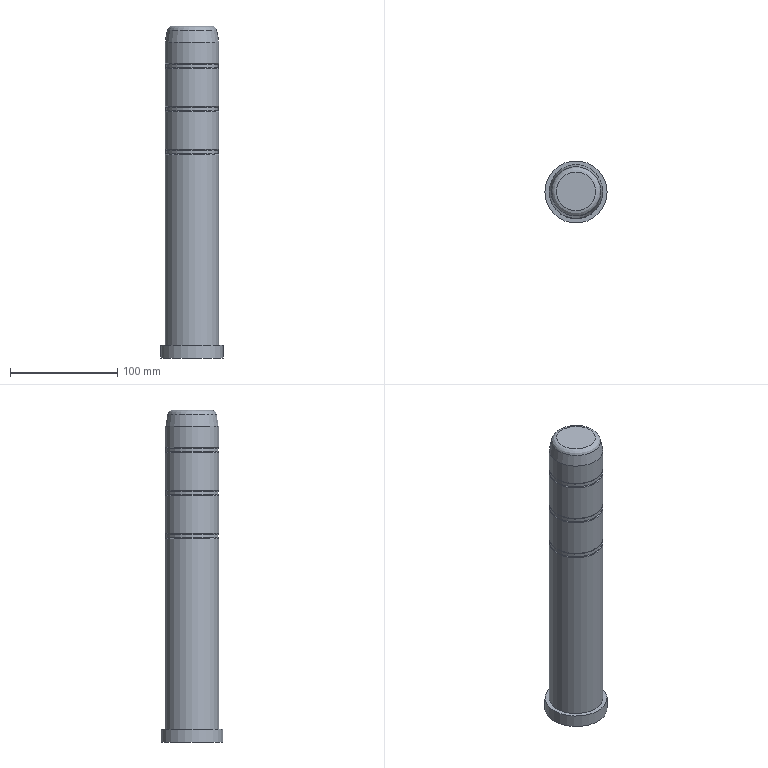Part | STEP file | GP50 | 1 solid | 19 faces | box 58 x 58 x 310 mm | volume 612293 mm3 | cylinder 8 | torus 7 | plane 3 | cone 1 | commonest cylinder face diameters 50 x4 49 x3 58 x1
STEP:
#1=CARTESIAN_POINT('',(0.,0.,0.));
#2=DIRECTION('',(0.,0.,1.));
#3=DIRECTION('',(1.,0.,0.));
#4=AXIS2_PLACEMENT_3D('',#1,#2,#3);
#5=CARTESIAN_POINT('',(247.,-268.,44.));
#6=VERTEX_POINT('',#5);
#7=CARTESIAN_POINT('',(222.,-268.,44.));
#8=DIRECTION('',(0.,0.,1.));
#9=DIRECTION('',(1.,0.,0.));
#10=AXIS2_PLACEMENT_3D('',#7,#8,#9);
#11=CIRCLE('',#10,25.);
#12=CARTESIAN_POINT('',(222.,-268.,534.));
#13=DIRECTION('',(0.,0.,-1.));
#14=DIRECTION('',(1.,0.,0.));
#15=AXIS2_PLACEMENT_3D('',#12,#13,#14);
#16=CYLINDRICAL_SURFACE('',#15,25.);
#17=CARTESIAN_POINT('',(6.283,490.));
#18=DIRECTION('',(-1.,0.));
#19=VECTOR('',#18,1.);
#20=LINE('',#17,#19);
#21=(GEOMETRIC_REPRESENTATION_CONTEXT(2)PARAMETRIC_REPRESENTATION_CONTEXT()REPRESENTATION_CONTEXT('',''));
#22=DEFINITIONAL_REPRESENTATION('',(#20),#21);
#23=PCURVE('',#16,#22);
#24=CARTESIAN_POINT('',(222.,-268.,43.134));
#25=DIRECTION('',(0.,0.,1.));
#26=DIRECTION('',(1.,0.,0.));
#27=AXIS2_PLACEMENT_3D('',#24,#25,#26);
#28=TOROIDAL_SURFACE('',#27,25.5,1.);
#29=CARTESIAN_POINT('',(0.,8.378));
#30=DIRECTION('',(1.,0.));
#31=VECTOR('',#30,1.);
#32=LINE('',#29,#31);
#33=(GEOMETRIC_REPRESENTATION_CONTEXT(2)PARAMETRIC_REPRESENTATION_CONTEXT()REPRESENTATION_CONTEXT('',''));
#34=DEFINITIONAL_REPRESENTATION('',(#32),#33);
#35=PCURVE('',#28,#34);
#36=SURFACE_CURVE('',#11,(#23,#35),.PCURVE_S1.);
#37=EDGE_CURVE('',#6,#6,#36,.T.);
#38=ORIENTED_EDGE('',*,*,#37,.T.);
#39=CARTESIAN_POINT('',(247.,-268.,79.));
#40=VERTEX_POINT('',#39);
#41=CARTESIAN_POINT('',(247.,-268.,79.));
#42=CARTESIAN_POINT('',(247.,-268.,44.));
#43=B_SPLINE_CURVE_WITH_KNOTS('',1,(#41,#42),.UNSPECIFIED.,.F.,.F.,(2,2),(455.,490.),.PIECEWISE_BEZIER_KNOTS.);
#44=CARTESIAN_POINT('',(0.,0.));
#45=DIRECTION('',(0.,1.));
#46=VECTOR('',#45,1.);
#47=LINE('',#44,#46);
#48=(GEOMETRIC_REPRESENTATION_CONTEXT(2)PARAMETRIC_REPRESENTATION_CONTEXT()REPRESENTATION_CONTEXT('',''));
#49=DEFINITIONAL_REPRESENTATION('',(#47),#48);
#50=PCURVE('',#16,#49);
#51=CARTESIAN_POINT('',(6.283,0.));
#52=DIRECTION('',(0.,1.));
#53=VECTOR('',#52,1.);
#54=LINE('',#51,#53);
#55=(GEOMETRIC_REPRESENTATION_CONTEXT(2)PARAMETRIC_REPRESENTATION_CONTEXT()REPRESENTATION_CONTEXT('',''));
#56=DEFINITIONAL_REPRESENTATION('',(#54),#55);
#57=PCURVE('',#16,#56);
#58=SEAM_CURVE('',#43,(#50,#57),.PCURVE_S1.);
#59=EDGE_CURVE('',#40,#6,#58,.T.);
#60=ORIENTED_EDGE('',*,*,#59,.F.);
#61=CARTESIAN_POINT('',(222.,-268.,79.));
#62=DIRECTION('',(0.,0.,1.));
#63=DIRECTION('',(1.,0.,0.));
#64=AXIS2_PLACEMENT_3D('',#61,#62,#63);
#65=CIRCLE('',#64,25.);
#66=CARTESIAN_POINT('',(6.283,455.));
#67=DIRECTION('',(-1.,0.));
#68=VECTOR('',#67,1.);
#69=LINE('',#66,#68);
#70=(GEOMETRIC_REPRESENTATION_CONTEXT(2)PARAMETRIC_REPRESENTATION_CONTEXT()REPRESENTATION_CONTEXT('',''));
#71=DEFINITIONAL_REPRESENTATION('',(#69),#70);
#72=PCURVE('',#16,#71);
#73=CARTESIAN_POINT('',(222.,-268.,79.866));
#74=DIRECTION('',(0.,0.,-1.));
#75=DIRECTION('',(-1.,0.,0.));
#76=AXIS2_PLACEMENT_3D('',#73,#74,#75);
#77=TOROIDAL_SURFACE('',#76,25.5,1.);
#78=CARTESIAN_POINT('',(9.425,8.378));
#79=DIRECTION('',(-1.,0.));
#80=VECTOR('',#79,1.);
#81=LINE('',#78,#80);
#82=(GEOMETRIC_REPRESENTATION_CONTEXT(2)PARAMETRIC_REPRESENTATION_CONTEXT()REPRESENTATION_CONTEXT('',''));
#83=DEFINITIONAL_REPRESENTATION('',(#81),#82);
#84=PCURVE('',#77,#83);
#85=SURFACE_CURVE('',#65,(#72,#84),.PCURVE_S1.);
#86=EDGE_CURVE('',#40,#40,#85,.T.);
#87=ORIENTED_EDGE('',*,*,#86,.F.);
#88=ORIENTED_EDGE('',*,*,#59,.T.);
#89=EDGE_LOOP('',(#38,#60,#87,#88));
#90=FACE_BOUND('',#89,.T.);
#91=ADVANCED_FACE('',(#90),#16,.T.);
#92=CARTESIAN_POINT('',(246.5,-268.,83.134));
#93=VERTEX_POINT('',#92);
#94=CARTESIAN_POINT('',(222.,-268.,83.134));
#95=DIRECTION('',(0.,0.,-1.));
#96=DIRECTION('',(1.,0.,0.));
#97=AXIS2_PLACEMENT_3D('',#94,#95,#96);
#98=CIRCLE('',#97,24.5);
#99=CARTESIAN_POINT('',(222.,-268.,534.));
#100=DIRECTION('',(0.,0.,-1.));
#101=DIRECTION('',(1.,0.,0.));
#102=AXIS2_PLACEMENT_3D('',#99,#100,#101);
#103=CYLINDRICAL_SURFACE('',#102,24.5);
#104=CARTESIAN_POINT('',(0.,450.866));
#105=DIRECTION('',(1.,0.));
#106=VECTOR('',#105,1.);
#107=LINE('',#104,#106);
#108=(GEOMETRIC_REPRESENTATION_CONTEXT(2)PARAMETRIC_REPRESENTATION_CONTEXT()REPRESENTATION_CONTEXT('',''));
#109=DEFINITIONAL_REPRESENTATION('',(#107),#108);
#110=PCURVE('',#103,#109);
#111=CARTESIAN_POINT('',(222.,-268.,83.134));
#112=DIRECTION('',(0.,0.,1.));
#113=DIRECTION('',(1.,0.,0.));
#114=AXIS2_PLACEMENT_3D('',#111,#112,#113);
#115=TOROIDAL_SURFACE('',#114,25.5,1.);
#116=CARTESIAN_POINT('',(6.283,9.425));
#117=DIRECTION('',(-1.,0.));
#118=VECTOR('',#117,1.);
#119=LINE('',#116,#118);
#120=(GEOMETRIC_REPRESENTATION_CONTEXT(2)PARAMETRIC_REPRESENTATION_CONTEXT()REPRESENTATION_CONTEXT('',''));
#121=DEFINITIONAL_REPRESENTATION('',(#119),#120);
#122=PCURVE('',#115,#121);
#123=SURFACE_CURVE('',#98,(#110,#122),.PCURVE_S1.);
#124=EDGE_CURVE('',#93,#93,#123,.T.);
#125=ORIENTED_EDGE('',*,*,#124,.T.);
#126=CARTESIAN_POINT('',(246.5,-268.,79.866));
#127=VERTEX_POINT('',#126);
#128=CARTESIAN_POINT('',(246.5,-268.,83.134));
#129=CARTESIAN_POINT('',(246.5,-268.,79.866));
#130=B_SPLINE_CURVE_WITH_KNOTS('',1,(#128,#129),.UNSPECIFIED.,.F.,.F.,(2,2),(450.866,454.134),.PIECEWISE_BEZIER_KNOTS.);
#131=CARTESIAN_POINT('',(6.283,0.));
#132=DIRECTION('',(0.,1.));
#133=VECTOR('',#132,1.);
#134=LINE('',#131,#133);
#135=(GEOMETRIC_REPRESENTATION_CONTEXT(2)PARAMETRIC_REPRESENTATION_CONTEXT()REPRESENTATION_CONTEXT('',''));
#136=DEFINITIONAL_REPRESENTATION('',(#134),#135);
#137=PCURVE('',#103,#136);
#138=CARTESIAN_POINT('',(0.,0.));
#139=DIRECTION('',(0.,1.));
#140=VECTOR('',#139,1.);
#141=LINE('',#138,#140);
#142=(GEOMETRIC_REPRESENTATION_CONTEXT(2)PARAMETRIC_REPRESENTATION_CONTEXT()REPRESENTATION_CONTEXT('',''));
#143=DEFINITIONAL_REPRESENTATION('',(#141),#142);
#144=PCURVE('',#103,#143);
#145=SEAM_CURVE('',#130,(#137,#144),.PCURVE_S1.);
#146=EDGE_CURVE('',#93,#127,#145,.T.);
#147=ORIENTED_EDGE('',*,*,#146,.T.);
#148=CARTESIAN_POINT('',(197.5,-268.,79.866));
#149=VERTEX_POINT('',#148);
#150=CARTESIAN_POINT('',(222.,-268.,79.866));
#151=DIRECTION('',(0.,0.,1.));
#152=DIRECTION('',(-1.,0.,0.));
#153=AXIS2_PLACEMENT_3D('',#150,#151,#152);
#154=CIRCLE('',#153,24.5);
#155=CARTESIAN_POINT('',(9.425,454.134));
#156=DIRECTION('',(-1.,0.));
#157=VECTOR('',#156,1.);
#158=LINE('',#155,#157);
#159=(GEOMETRIC_REPRESENTATION_CONTEXT(2)PARAMETRIC_REPRESENTATION_CONTEXT()REPRESENTATION_CONTEXT('',''));
#160=DEFINITIONAL_REPRESENTATION('',(#158),#159);
#161=PCURVE('',#103,#160);
#162=CARTESIAN_POINT('',(12.566,9.425));
#163=DIRECTION('',(-1.,0.));
#164=VECTOR('',#163,1.);
#165=LINE('',#162,#164);
#166=(GEOMETRIC_REPRESENTATION_CONTEXT(2)PARAMETRIC_REPRESENTATION_CONTEXT()REPRESENTATION_CONTEXT('',''));
#167=DEFINITIONAL_REPRESENTATION('',(#165),#166);
#168=PCURVE('',#77,#167);
#169=SURFACE_CURVE('',#154,(#161,#168),.PCURVE_S1.);
#170=EDGE_CURVE('',#127,#149,#169,.T.);
#171=ORIENTED_EDGE('',*,*,#170,.T.);
#172=CARTESIAN_POINT('',(222.,-268.,79.866));
#173=DIRECTION('',(0.,0.,1.));
#174=DIRECTION('',(-1.,0.,0.));
#175=AXIS2_PLACEMENT_3D('',#172,#173,#174);
#176=CIRCLE('',#175,24.5);
#177=CARTESIAN_POINT('',(3.142,454.134));
#178=DIRECTION('',(-1.,0.));
#179=VECTOR('',#178,1.);
#180=LINE('',#177,#179);
#181=(GEOMETRIC_REPRESENTATION_CONTEXT(2)PARAMETRIC_REPRESENTATION_CONTEXT()REPRESENTATION_CONTEXT('',''));
#182=DEFINITIONAL_REPRESENTATION('',(#180),#181);
#183=PCURVE('',#103,#182);
#184=CARTESIAN_POINT('',(6.283,9.425));
#185=DIRECTION('',(-1.,0.));
#186=VECTOR('',#185,1.);
#187=LINE('',#184,#186);
#188=(GEOMETRIC_REPRESENTATION_CONTEXT(2)PARAMETRIC_REPRESENTATION_CONTEXT()REPRESENTATION_CONTEXT('',''));
#189=DEFINITIONAL_REPRESENTATION('',(#187),#188);
#190=PCURVE('',#77,#189);
#191=SURFACE_CURVE('',#176,(#183,#190),.PCURVE_S1.);
#192=EDGE_CURVE('',#149,#127,#191,.T.);
#193=ORIENTED_EDGE('',*,*,#192,.T.);
#194=ORIENTED_EDGE('',*,*,#146,.F.);
#195=EDGE_LOOP('',(#125,#147,#171,#193,#194));
#196=FACE_BOUND('',#195,.T.);
#197=ADVANCED_FACE('',(#196),#103,.T.);
#198=CARTESIAN_POINT('',(246.5,-268.,123.134));
#199=VERTEX_POINT('',#198);
#200=CARTESIAN_POINT('',(222.,-268.,123.134));
#201=DIRECTION('',(0.,0.,-1.));
#202=DIRECTION('',(1.,0.,0.));
#203=AXIS2_PLACEMENT_3D('',#200,#201,#202);
#204=CIRCLE('',#203,24.5);
#205=CARTESIAN_POINT('',(222.,-268.,534.));
#206=DIRECTION('',(0.,0.,-1.));
#207=DIRECTION('',(1.,0.,0.));
#208=AXIS2_PLACEMENT_3D('',#205,#206,#207);
#209=CYLINDRICAL_SURFACE('',#208,24.5);
#210=CARTESIAN_POINT('',(0.,410.866));
#211=DIRECTION('',(1.,0.));
#212=VECTOR('',#211,1.);
#213=LINE('',#210,#212);
#214=(GEOMETRIC_REPRESENTATION_CONTEXT(2)PARAMETRIC_REPRESENTATION_CONTEXT()REPRESENTATION_CONTEXT('',''));
#215=DEFINITIONAL_REPRESENTATION('',(#213),#214);
#216=PCURVE('',#209,#215);
#217=CARTESIAN_POINT('',(222.,-268.,123.134));
#218=DIRECTION('',(0.,0.,1.));
#219=DIRECTION('',(1.,0.,0.));
#220=AXIS2_PLACEMENT_3D('',#217,#218,#219);
#221=TOROIDAL_SURFACE('',#220,25.5,1.);
#222=CARTESIAN_POINT('',(6.283,9.425));
#223=DIRECTION('',(-1.,0.));
#224=VECTOR('',#223,1.);
#225=LINE('',#222,#224);
#226=(GEOMETRIC_REPRESENTATION_CONTEXT(2)PARAMETRIC_REPRESENTATION_CONTEXT()REPRESENTATION_CONTEXT('',''));
#227=DEFINITIONAL_REPRESENTATION('',(#225),#226);
#228=PCURVE('',#221,#227);
#229=SURFACE_CURVE('',#204,(#216,#228),.PCURVE_S1.);
#230=EDGE_CURVE('',#199,#199,#229,.T.);
#231=ORIENTED_EDGE('',*,*,#230,.T.);
#232=CARTESIAN_POINT('',(246.5,-268.,119.866));
#233=VERTEX_POINT('',#232);
#234=CARTESIAN_POINT('',(246.5,-268.,123.134));
#235=CARTESIAN_POINT('',(246.5,-268.,119.866));
#236=B_SPLINE_CURVE_WITH_KNOTS('',1,(#234,#235),.UNSPECIFIED.,.F.,.F.,(2,2),(410.866,414.134),.PIECEWISE_BEZIER_KNOTS.);
#237=CARTESIAN_POINT('',(6.283,0.));
#238=DIRECTION('',(0.,1.));
#239=VECTOR('',#238,1.);
#240=LINE('',#237,#239);
#241=(GEOMETRIC_REPRESENTATION_CONTEXT(2)PARAMETRIC_REPRESENTATION_CONTEXT()REPRESENTATION_CONTEXT('',''));
#242=DEFINITIONAL_REPRESENTATION('',(#240),#241);
#243=PCURVE('',#209,#242);
#244=CARTESIAN_POINT('',(0.,0.));
#245=DIRECTION('',(0.,1.));
#246=VECTOR('',#245,1.);
#247=LINE('',#244,#246);
#248=(GEOMETRIC_REPRESENTATION_CONTEXT(2)PARAMETRIC_REPRESENTATION_CONTEXT()REPRESENTATION_CONTEXT('',''));
#249=DEFINITIONAL_REPRESENTATION('',(#247),#248);
#250=PCURVE('',#209,#249);
#251=SEAM_CURVE('',#236,(#243,#250),.PCURVE_S1.);
#252=EDGE_CURVE('',#199,#233,#251,.T.);
#253=ORIENTED_EDGE('',*,*,#252,.T.);
#254=CARTESIAN_POINT('',(197.5,-268.,119.866));
#255=VERTEX_POINT('',#254);
#256=CARTESIAN_POINT('',(222.,-268.,119.866));
#257=DIRECTION('',(0.,0.,1.));
#258=DIRECTION('',(-1.,0.,0.));
#259=AXIS2_PLACEMENT_3D('',#256,#257,#258);
#260=CIRCLE('',#259,24.5);
#261=CARTESIAN_POINT('',(9.425,414.134));
#262=DIRECTION('',(-1.,0.));
#263=VECTOR('',#262,1.);
#264=LINE('',#261,#263);
#265=(GEOMETRIC_REPRESENTATION_CONTEXT(2)PARAMETRIC_REPRESENTATION_CONTEXT()REPRESENTATION_CONTEXT('',''));
#266=DEFINITIONAL_REPRESENTATION('',(#264),#265);
#267=PCURVE('',#209,#266);
#268=CARTESIAN_POINT('',(222.,-268.,119.866));
#269=DIRECTION('',(0.,0.,-1.));
#270=DIRECTION('',(-1.,0.,0.));
#271=AXIS2_PLACEMENT_3D('',#268,#269,#270);
#272=TOROIDAL_SURFACE('',#271,25.5,1.);
#273=CARTESIAN_POINT('',(12.566,9.425));
#274=DIRECTION('',(-1.,0.));
#275=VECTOR('',#274,1.);
#276=LINE('',#273,#275);
#277=(GEOMETRIC_REPRESENTATION_CONTEXT(2)PARAMETRIC_REPRESENTATION_CONTEXT()REPRESENTATION_CONTEXT('',''));
#278=DEFINITIONAL_REPRESENTATION('',(#276),#277);
#279=PCURVE('',#272,#278);
#280=SURFACE_CURVE('',#260,(#267,#279),.PCURVE_S1.);
#281=EDGE_CURVE('',#233,#255,#280,.T.);
#282=ORIENTED_EDGE('',*,*,#281,.T.);
#283=CARTESIAN_POINT('',(222.,-268.,119.866));
#284=DIRECTION('',(0.,0.,1.));
#285=DIRECTION('',(-1.,0.,0.));
#286=AXIS2_PLACEMENT_3D('',#283,#284,#285);
#287=CIRCLE('',#286,24.5);
#288=CARTESIAN_POINT('',(3.142,414.134));
#289=DIRECTION('',(-1.,0.));
#290=VECTOR('',#289,1.);
#291=LINE('',#288,#290);
#292=(GEOMETRIC_REPRESENTATION_CONTEXT(2)PARAMETRIC_REPRESENTATION_CONTEXT()REPRESENTATION_CONTEXT('',''));
#293=DEFINITIONAL_REPRESENTATION('',(#291),#292);
#294=PCURVE('',#209,#293);
#295=CARTESIAN_POINT('',(6.283,9.425));
#296=DIRECTION('',(-1.,0.));
#297=VECTOR('',#296,1.);
#298=LINE('',#295,#297);
#299=(GEOMETRIC_REPRESENTATION_CONTEXT(2)PARAMETRIC_REPRESENTATION_CONTEXT()REPRESENTATION_CONTEXT('',''));
#300=DEFINITIONAL_REPRESENTATION('',(#298),#299);
#301=PCURVE('',#272,#300);
#302=SURFACE_CURVE('',#287,(#294,#301),.PCURVE_S1.);
#303=EDGE_CURVE('',#255,#233,#302,.T.);
#304=ORIENTED_EDGE('',*,*,#303,.T.);
#305=ORIENTED_EDGE('',*,*,#252,.F.);
#306=EDGE_LOOP('',(#231,#253,#282,#304,#305));
#307=FACE_BOUND('',#306,.T.);
#308=ADVANCED_FACE('',(#307),#209,.T.);
#309=CARTESIAN_POINT('',(203.84,-268.,159.));
#310=VERTEX_POINT('',#309);
#311=CARTESIAN_POINT('',(222.,-268.,159.));
#312=DIRECTION('',(0.,0.,1.));
#313=DIRECTION('',(-1.,0.,0.));
#314=AXIS2_PLACEMENT_3D('',#311,#312,#313);
#315=CIRCLE('',#314,18.16);
#316=CARTESIAN_POINT('',(-222.,272.,159.));
#317=DIRECTION('',(0.,0.,-1.));
#318=DIRECTION('',(1.,0.,0.));
#319=AXIS2_PLACEMENT_3D('',#316,#317,#318);
#320=PLANE('',#319);
#321=CARTESIAN_POINT('',(425.84,540.));
#322=CARTESIAN_POINT('',(425.84,571.453));
#323=CARTESIAN_POINT('',(453.08,555.727));
#324=CARTESIAN_POINT('',(480.319,540.));
#325=CARTESIAN_POINT('',(453.08,524.273));
#326=CARTESIAN_POINT('',(425.84,508.547));
#327=CARTESIAN_POINT('',(425.84,540.));
#328=(BOUNDED_CURVE()B_SPLINE_CURVE(2,(#321,#322,#323,#324,#325,#326,#327),.UNSPECIFIED.,.T.,.F.)B_SPLINE_CURVE_WITH_KNOTS((1,2,2,2,2,1),(-2.094,0.,2.094,4.189,6.283,8.378),.UNSPECIFIED.)CURVE()GEOMETRIC_REPRESENTATION_ITEM()RATIONAL_B_SPLINE_CURVE((1.,0.5,1.,0.5,1.,0.5,1.))REPRESENTATION_ITEM(''));
#329=(GEOMETRIC_REPRESENTATION_CONTEXT(2)PARAMETRIC_REPRESENTATION_CONTEXT()REPRESENTATION_CONTEXT('',''));
#330=DEFINITIONAL_REPRESENTATION('',(#328),#329);
#331=PCURVE('',#320,#330);
#332=CARTESIAN_POINT('',(222.,-268.,154.));
#333=DIRECTION('',(0.,0.,-1.));
#334=DIRECTION('',(-1.,0.,0.));
#335=AXIS2_PLACEMENT_3D('',#332,#333,#334);
#336=TOROIDAL_SURFACE('',#335,18.16,5.);
#337=CARTESIAN_POINT('',(6.283,4.712));
#338=DIRECTION('',(-1.,0.));
#339=VECTOR('',#338,1.);
#340=LINE('',#337,#339);
#341=(GEOMETRIC_REPRESENTATION_CONTEXT(2)PARAMETRIC_REPRESENTATION_CONTEXT()REPRESENTATION_CONTEXT('',''));
#342=DEFINITIONAL_REPRESENTATION('',(#340),#341);
#343=PCURVE('',#336,#342);
#344=SURFACE_CURVE('',#315,(#331,#343),.PCURVE_S1.);
#345=EDGE_CURVE('',#310,#310,#344,.T.);
#346=ORIENTED_EDGE('',*,*,#345,.T.);
#347=EDGE_LOOP('',(#346));
#348=FACE_BOUND('',#347,.T.);
#349=ADVANCED_FACE('',(#348),#320,.F.);
#350=CARTESIAN_POINT('',(198.916,-268.,154.868));
#351=VERTEX_POINT('',#350);
#352=CARTESIAN_POINT('',(222.,-268.,154.868));
#353=DIRECTION('',(0.,0.,-1.));
#354=DIRECTION('',(-1.,0.,0.));
#355=AXIS2_PLACEMENT_3D('',#352,#353,#354);
#356=CIRCLE('',#355,23.084);
#357=CARTESIAN_POINT('',(0.,6.109));
#358=DIRECTION('',(1.,0.));
#359=VECTOR('',#358,1.);
#360=LINE('',#357,#359);
#361=(GEOMETRIC_REPRESENTATION_CONTEXT(2)PARAMETRIC_REPRESENTATION_CONTEXT()REPRESENTATION_CONTEXT('',''));
#362=DEFINITIONAL_REPRESENTATION('',(#360),#361);
#363=PCURVE('',#336,#362);
#364=CARTESIAN_POINT('',(222.,-268.,159.));
#365=DIRECTION('',(0.,0.,-1.));
#366=DIRECTION('',(-1.,0.,0.));
#367=AXIS2_PLACEMENT_3D('',#364,#365,#366);
#368=CONICAL_SURFACE('',#367,22.355,0.1745);
#369=CARTESIAN_POINT('',(0.,4.132));
#370=DIRECTION('',(1.,0.));
#371=VECTOR('',#370,1.);
#372=LINE('',#369,#371);
#373=(GEOMETRIC_REPRESENTATION_CONTEXT(2)PARAMETRIC_REPRESENTATION_CONTEXT()REPRESENTATION_CONTEXT('',''));
#374=DEFINITIONAL_REPRESENTATION('',(#372),#373);
#375=PCURVE('',#368,#374);
#376=SURFACE_CURVE('',#356,(#363,#375),.PCURVE_S1.);
#377=EDGE_CURVE('',#351,#351,#376,.T.);
#378=ORIENTED_EDGE('',*,*,#377,.F.);
#379=CARTESIAN_POINT('',(203.84,-268.,159.));
#380=CARTESIAN_POINT('',(202.658,-268.,159.));
#381=CARTESIAN_POINT('',(201.499,-268.,158.667));
#382=CARTESIAN_POINT('',(200.466,-268.,158.021));
#383=CARTESIAN_POINT('',(199.651,-268.,157.116));
#384=CARTESIAN_POINT('',(199.122,-268.,156.033));
#385=CARTESIAN_POINT('',(198.916,-268.,154.868));
#386=(BOUNDED_CURVE()B_SPLINE_CURVE(6,(#379,#380,#381,#382,#383,#384,#385),.UNSPECIFIED.,.F.,.F.)B_SPLINE_CURVE_WITH_KNOTS((7,7),(4.712,6.109),.PIECEWISE_BEZIER_KNOTS.)CURVE()GEOMETRIC_REPRESENTATION_ITEM()RATIONAL_B_SPLINE_CURVE((1.025,1.008,0.9984,0.9952,0.9984,1.008,1.025))REPRESENTATION_ITEM(''));
#387=CARTESIAN_POINT('',(0.,0.));
#388=DIRECTION('',(0.,1.));
#389=VECTOR('',#388,1.);
#390=LINE('',#387,#389);
#391=(GEOMETRIC_REPRESENTATION_CONTEXT(2)PARAMETRIC_REPRESENTATION_CONTEXT()REPRESENTATION_CONTEXT('',''));
#392=DEFINITIONAL_REPRESENTATION('',(#390),#391);
#393=PCURVE('',#336,#392);
#394=CARTESIAN_POINT('',(6.283,0.));
#395=DIRECTION('',(0.,1.));
#396=VECTOR('',#395,1.);
#397=LINE('',#394,#396);
#398=(GEOMETRIC_REPRESENTATION_CONTEXT(2)PARAMETRIC_REPRESENTATION_CONTEXT()REPRESENTATION_CONTEXT('',''));
#399=DEFINITIONAL_REPRESENTATION('',(#397),#398);
#400=PCURVE('',#336,#399);
#401=SEAM_CURVE('',#386,(#393,#400),.PCURVE_S1.);
#402=EDGE_CURVE('',#310,#351,#401,.T.);
#403=ORIENTED_EDGE('',*,*,#402,.F.);
#404=ORIENTED_EDGE('',*,*,#345,.F.);
#405=ORIENTED_EDGE('',*,*,#402,.T.);
#406=EDGE_LOOP('',(#378,#403,#404,#405));
#407=FACE_BOUND('',#406,.T.);
#408=ADVANCED_FACE('',(#407),#336,.T.);
#409=ORIENTED_EDGE('',*,*,#377,.T.);
#410=CARTESIAN_POINT('',(197.,-268.,144.));
#411=VERTEX_POINT('',#410);
#412=CARTESIAN_POINT('',(198.916,-268.,154.868));
#413=CARTESIAN_POINT('',(197.,-268.,144.));
#414=B_SPLINE_CURVE_WITH_KNOTS('',1,(#412,#413),.UNSPECIFIED.,.F.,.F.,(2,2),(4.195,15.231),.PIECEWISE_BEZIER_KNOTS.);
#415=CARTESIAN_POINT('',(6.283,0.));
#416=DIRECTION('',(0.,1.));
#417=VECTOR('',#416,1.);
#418=LINE('',#415,#417);
#419=(GEOMETRIC_REPRESENTATION_CONTEXT(2)PARAMETRIC_REPRESENTATION_CONTEXT()REPRESENTATION_CONTEXT('',''));
#420=DEFINITIONAL_REPRESENTATION('',(#418),#419);
#421=PCURVE('',#368,#420);
#422=CARTESIAN_POINT('',(0.,0.));
#423=DIRECTION('',(0.,1.));
#424=VECTOR('',#423,1.);
#425=LINE('',#422,#424);
#426=(GEOMETRIC_REPRESENTATION_CONTEXT(2)PARAMETRIC_REPRESENTATION_CONTEXT()REPRESENTATION_CONTEXT('',''));
#427=DEFINITIONAL_REPRESENTATION('',(#425),#426);
#428=PCURVE('',#368,#427);
#429=SEAM_CURVE('',#414,(#421,#428),.PCURVE_S1.);
#430=EDGE_CURVE('',#351,#411,#429,.T.);
#431=ORIENTED_EDGE('',*,*,#430,.T.);
#432=CARTESIAN_POINT('',(247.,-268.,144.));
#433=VERTEX_POINT('',#432);
#434=CARTESIAN_POINT('',(222.,-268.,144.));
#435=DIRECTION('',(0.,0.,-1.));
#436=DIRECTION('',(-1.,0.,0.));
#437=AXIS2_PLACEMENT_3D('',#434,#435,#436);
#438=CIRCLE('',#437,25.);
#439=CARTESIAN_POINT('',(0.,15.));
#440=DIRECTION('',(1.,0.));
#441=VECTOR('',#440,1.);
#442=LINE('',#439,#441);
#443=(GEOMETRIC_REPRESENTATION_CONTEXT(2)PARAMETRIC_REPRESENTATION_CONTEXT()REPRESENTATION_CONTEXT('',''));
#444=DEFINITIONAL_REPRESENTATION('',(#442),#443);
#445=PCURVE('',#368,#444);
#446=CARTESIAN_POINT('',(222.,-268.,534.));
#447=DIRECTION('',(0.,0.,-1.));
#448=DIRECTION('',(1.,0.,0.));
#449=AXIS2_PLACEMENT_3D('',#446,#447,#448);
#450=CYLINDRICAL_SURFACE('',#449,25.);
#451=CARTESIAN_POINT('',(-3.142,390.));
#452=DIRECTION('',(1.,0.));
#453=VECTOR('',#452,1.);
#454=LINE('',#451,#453);
#455=(GEOMETRIC_REPRESENTATION_CONTEXT(2)PARAMETRIC_REPRESENTATION_CONTEXT()REPRESENTATION_CONTEXT('',''));
#456=DEFINITIONAL_REPRESENTATION('',(#454),#455);
#457=PCURVE('',#450,#456);
#458=SURFACE_CURVE('',#438,(#445,#457),.PCURVE_S1.);
#459=EDGE_CURVE('',#433,#411,#458,.T.);
#460=ORIENTED_EDGE('',*,*,#459,.F.);
#461=CARTESIAN_POINT('',(222.,-268.,144.));
#462=DIRECTION('',(0.,0.,-1.));
#463=DIRECTION('',(-1.,0.,0.));
#464=AXIS2_PLACEMENT_3D('',#461,#462,#463);
#465=CIRCLE('',#464,25.);
#466=CARTESIAN_POINT('',(0.,15.));
#467=DIRECTION('',(1.,0.));
#468=VECTOR('',#467,1.);
#469=LINE('',#466,#468);
#470=(GEOMETRIC_REPRESENTATION_CONTEXT(2)PARAMETRIC_REPRESENTATION_CONTEXT()REPRESENTATION_CONTEXT('',''));
#471=DEFINITIONAL_REPRESENTATION('',(#469),#470);
#472=PCURVE('',#368,#471);
#473=CARTESIAN_POINT('',(3.142,390.));
#474=DIRECTION('',(1.,0.));
#475=VECTOR('',#474,1.);
#476=LINE('',#473,#475);
#477=(GEOMETRIC_REPRESENTATION_CONTEXT(2)PARAMETRIC_REPRESENTATION_CONTEXT()REPRESENTATION_CONTEXT('',''));
#478=DEFINITIONAL_REPRESENTATION('',(#476),#477);
#479=PCURVE('',#450,#478);
#480=SURFACE_CURVE('',#465,(#472,#479),.PCURVE_S1.);
#481=EDGE_CURVE('',#411,#433,#480,.T.);
#482=ORIENTED_EDGE('',*,*,#481,.F.);
#483=ORIENTED_EDGE('',*,*,#430,.F.);
#484=EDGE_LOOP('',(#409,#431,#460,#482,#483));
#485=FACE_BOUND('',#484,.T.);
#486=ADVANCED_FACE('',(#485),#368,.T.);
#487=CARTESIAN_POINT('',(247.,-268.,124.));
#488=VERTEX_POINT('',#487);
#489=CARTESIAN_POINT('',(222.,-268.,124.));
#490=DIRECTION('',(0.,0.,1.));
#491=DIRECTION('',(1.,0.,0.));
#492=AXIS2_PLACEMENT_3D('',#489,#490,#491);
#493=CIRCLE('',#492,25.);
#494=CARTESIAN_POINT('',(6.283,410.));
#495=DIRECTION('',(-1.,0.));
#496=VECTOR('',#495,1.);
#497=LINE('',#494,#496);
#498=(GEOMETRIC_REPRESENTATION_CONTEXT(2)PARAMETRIC_REPRESENTATION_CONTEXT()REPRESENTATION_CONTEXT('',''));
#499=DEFINITIONAL_REPRESENTATION('',(#497),#498);
#500=PCURVE('',#450,#499);
#501=CARTESIAN_POINT('',(0.,8.378));
#502=DIRECTION('',(1.,0.));
#503=VECTOR('',#502,1.);
#504=LINE('',#501,#503);
#505=(GEOMETRIC_REPRESENTATION_CONTEXT(2)PARAMETRIC_REPRESENTATION_CONTEXT()REPRESENTATION_CONTEXT('',''));
#506=DEFINITIONAL_REPRESENTATION('',(#504),#505);
#507=PCURVE('',#221,#506);
#508=SURFACE_CURVE('',#493,(#500,#507),.PCURVE_S1.);
#509=EDGE_CURVE('',#488,#488,#508,.T.);
#510=ORIENTED_EDGE('',*,*,#509,.T.);
#511=CARTESIAN_POINT('',(247.,-268.,144.));
#512=CARTESIAN_POINT('',(247.,-268.,124.));
#513=B_SPLINE_CURVE_WITH_KNOTS('',1,(#511,#512),.UNSPECIFIED.,.F.,.F.,(2,2),(390.,410.),.PIECEWISE_BEZIER_KNOTS.);
#514=CARTESIAN_POINT('',(0.,0.));
#515=DIRECTION('',(0.,1.));
#516=VECTOR('',#515,1.);
#517=LINE('',#514,#516);
#518=(GEOMETRIC_REPRESENTATION_CONTEXT(2)PARAMETRIC_REPRESENTATION_CONTEXT()REPRESENTATION_CONTEXT('',''));
#519=DEFINITIONAL_REPRESENTATION('',(#517),#518);
#520=PCURVE('',#450,#519);
#521=CARTESIAN_POINT('',(6.283,0.));
#522=DIRECTION('',(0.,1.));
#523=VECTOR('',#522,1.);
#524=LINE('',#521,#523);
#525=(GEOMETRIC_REPRESENTATION_CONTEXT(2)PARAMETRIC_REPRESENTATION_CONTEXT()REPRESENTATION_CONTEXT('',''));
#526=DEFINITIONAL_REPRESENTATION('',(#524),#525);
#527=PCURVE('',#450,#526);
#528=SEAM_CURVE('',#513,(#520,#527),.PCURVE_S1.);
#529=EDGE_CURVE('',#433,#488,#528,.T.);
#530=ORIENTED_EDGE('',*,*,#529,.F.);
#531=ORIENTED_EDGE('',*,*,#459,.T.);
#532=ORIENTED_EDGE('',*,*,#481,.T.);
#533=ORIENTED_EDGE('',*,*,#529,.T.);
#534=EDGE_LOOP('',(#510,#530,#531,#532,#533));
#535=FACE_BOUND('',#534,.T.);
#536=ADVANCED_FACE('',(#535),#450,.T.);
#537=CARTESIAN_POINT('',(247.,-268.,84.));
#538=VERTEX_POINT('',#537);
#539=CARTESIAN_POINT('',(222.,-268.,84.));
#540=DIRECTION('',(0.,0.,1.));
#541=DIRECTION('',(1.,0.,0.));
#542=AXIS2_PLACEMENT_3D('',#539,#540,#541);
#543=CIRCLE('',#542,25.);
#544=CARTESIAN_POINT('',(222.,-268.,534.));
#545=DIRECTION('',(0.,0.,-1.));
#546=DIRECTION('',(1.,0.,0.));
#547=AXIS2_PLACEMENT_3D('',#544,#545,#546);
#548=CYLINDRICAL_SURFACE('',#547,25.);
#549=CARTESIAN_POINT('',(6.283,450.));
#550=DIRECTION('',(-1.,0.));
#551=VECTOR('',#550,1.);
#552=LINE('',#549,#551);
#553=(GEOMETRIC_REPRESENTATION_CONTEXT(2)PARAMETRIC_REPRESENTATION_CONTEXT()REPRESENTATION_CONTEXT('',''));
#554=DEFINITIONAL_REPRESENTATION('',(#552),#553);
#555=PCURVE('',#548,#554);
#556=CARTESIAN_POINT('',(0.,8.378));
#557=DIRECTION('',(1.,0.));
#558=VECTOR('',#557,1.);
#559=LINE('',#556,#558);
#560=(GEOMETRIC_REPRESENTATION_CONTEXT(2)PARAMETRIC_REPRESENTATION_CONTEXT()REPRESENTATION_CONTEXT('',''));
#561=DEFINITIONAL_REPRESENTATION('',(#559),#560);
#562=PCURVE('',#115,#561);
#563=SURFACE_CURVE('',#543,(#555,#562),.PCURVE_S1.);
#564=EDGE_CURVE('',#538,#538,#563,.T.);
#565=ORIENTED_EDGE('',*,*,#564,.T.);
#566=CARTESIAN_POINT('',(247.,-268.,119.));
#567=VERTEX_POINT('',#566);
#568=CARTESIAN_POINT('',(247.,-268.,119.));
#569=CARTESIAN_POINT('',(247.,-268.,84.));
#570=B_SPLINE_CURVE_WITH_KNOTS('',1,(#568,#569),.UNSPECIFIED.,.F.,.F.,(2,2),(415.,450.),.PIECEWISE_BEZIER_KNOTS.);
#571=CARTESIAN_POINT('',(0.,0.));
#572=DIRECTION('',(0.,1.));
#573=VECTOR('',#572,1.);
#574=LINE('',#571,#573);
#575=(GEOMETRIC_REPRESENTATION_CONTEXT(2)PARAMETRIC_REPRESENTATION_CONTEXT()REPRESENTATION_CONTEXT('',''));
#576=DEFINITIONAL_REPRESENTATION('',(#574),#575);
#577=PCURVE('',#548,#576);
#578=CARTESIAN_POINT('',(6.283,0.));
#579=DIRECTION('',(0.,1.));
#580=VECTOR('',#579,1.);
#581=LINE('',#578,#580);
#582=(GEOMETRIC_REPRESENTATION_CONTEXT(2)PARAMETRIC_REPRESENTATION_CONTEXT()REPRESENTATION_CONTEXT('',''));
#583=DEFINITIONAL_REPRESENTATION('',(#581),#582);
#584=PCURVE('',#548,#583);
#585=SEAM_CURVE('',#570,(#577,#584),.PCURVE_S1.);
#586=EDGE_CURVE('',#567,#538,#585,.T.);
#587=ORIENTED_EDGE('',*,*,#586,.F.);
#588=CARTESIAN_POINT('',(222.,-268.,119.));
#589=DIRECTION('',(0.,0.,1.));
#590=DIRECTION('',(1.,0.,0.));
#591=AXIS2_PLACEMENT_3D('',#588,#589,#590);
#592=CIRCLE('',#591,25.);
#593=CARTESIAN_POINT('',(6.283,415.));
#594=DIRECTION('',(-1.,0.));
#595=VECTOR('',#594,1.);
#596=LINE('',#593,#595);
#597=(GEOMETRIC_REPRESENTATION_CONTEXT(2)PARAMETRIC_REPRESENTATION_CONTEXT()REPRESENTATION_CONTEXT('',''));
#598=DEFINITIONAL_REPRESENTATION('',(#596),#597);
#599=PCURVE('',#548,#598);
#600=CARTESIAN_POINT('',(9.425,8.378));
#601=DIRECTION('',(-1.,0.));
#602=VECTOR('',#601,1.);
#603=LINE('',#600,#602);
#604=(GEOMETRIC_REPRESENTATION_CONTEXT(2)PARAMETRIC_REPRESENTATION_CONTEXT()REPRESENTATION_CONTEXT('',''));
#605=DEFINITIONAL_REPRESENTATION('',(#603),#604);
#606=PCURVE('',#272,#605);
#607=SURFACE_CURVE('',#592,(#599,#606),.PCURVE_S1.);
#608=EDGE_CURVE('',#567,#567,#607,.T.);
#609=ORIENTED_EDGE('',*,*,#608,.F.);
#610=ORIENTED_EDGE('',*,*,#586,.T.);
#611=EDGE_LOOP('',(#565,#587,#609,#610));
#612=FACE_BOUND('',#611,.T.);
#613=ADVANCED_FACE('',(#612),#548,.T.);
#614=CARTESIAN_POINT('',(246.5,-268.,43.134));
#615=VERTEX_POINT('',#614);
#616=CARTESIAN_POINT('',(222.,-268.,43.134));
#617=DIRECTION('',(0.,0.,-1.));
#618=DIRECTION('',(1.,0.,0.));
#619=AXIS2_PLACEMENT_3D('',#616,#617,#618);
#620=CIRCLE('',#619,24.5);
#621=CARTESIAN_POINT('',(222.,-268.,534.));
#622=DIRECTION('',(0.,0.,-1.));
#623=DIRECTION('',(1.,0.,0.));
#624=AXIS2_PLACEMENT_3D('',#621,#622,#623);
#625=CYLINDRICAL_SURFACE('',#624,24.5);
#626=CARTESIAN_POINT('',(0.,490.866));
#627=DIRECTION('',(1.,0.));
#628=VECTOR('',#627,1.);
#629=LINE('',#626,#628);
#630=(GEOMETRIC_REPRESENTATION_CONTEXT(2)PARAMETRIC_REPRESENTATION_CONTEXT()REPRESENTATION_CONTEXT('',''));
#631=DEFINITIONAL_REPRESENTATION('',(#629),#630);
#632=PCURVE('',#625,#631);
#633=CARTESIAN_POINT('',(6.283,9.425));
#634=DIRECTION('',(-1.,0.));
#635=VECTOR('',#634,1.);
#636=LINE('',#633,#635);
#637=(GEOMETRIC_REPRESENTATION_CONTEXT(2)PARAMETRIC_REPRESENTATION_CONTEXT()REPRESENTATION_CONTEXT('',''));
#638=DEFINITIONAL_REPRESENTATION('',(#636),#637);
#639=PCURVE('',#28,#638);
#640=SURFACE_CURVE('',#620,(#632,#639),.PCURVE_S1.);
#641=EDGE_CURVE('',#615,#615,#640,.T.);
#642=ORIENTED_EDGE('',*,*,#641,.T.);
#643=CARTESIAN_POINT('',(246.5,-268.,39.866));
#644=VERTEX_POINT('',#643);
#645=CARTESIAN_POINT('',(246.5,-268.,43.134));
#646=CARTESIAN_POINT('',(246.5,-268.,39.866));
#647=B_SPLINE_CURVE_WITH_KNOTS('',1,(#645,#646),.UNSPECIFIED.,.F.,.F.,(2,2),(490.866,494.134),.PIECEWISE_BEZIER_KNOTS.);
#648=CARTESIAN_POINT('',(6.283,0.));
#649=DIRECTION('',(0.,1.));
#650=VECTOR('',#649,1.);
#651=LINE('',#648,#650);
#652=(GEOMETRIC_REPRESENTATION_CONTEXT(2)PARAMETRIC_REPRESENTATION_CONTEXT()REPRESENTATION_CONTEXT('',''));
#653=DEFINITIONAL_REPRESENTATION('',(#651),#652);
#654=PCURVE('',#625,#653);
#655=CARTESIAN_POINT('',(0.,0.));
#656=DIRECTION('',(0.,1.));
#657=VECTOR('',#656,1.);
#658=LINE('',#655,#657);
#659=(GEOMETRIC_REPRESENTATION_CONTEXT(2)PARAMETRIC_REPRESENTATION_CONTEXT()REPRESENTATION_CONTEXT('',''));
#660=DEFINITIONAL_REPRESENTATION('',(#658),#659);
#661=PCURVE('',#625,#660);
#662=SEAM_CURVE('',#647,(#654,#661),.PCURVE_S1.);
#663=EDGE_CURVE('',#615,#644,#662,.T.);
#664=ORIENTED_EDGE('',*,*,#663,.T.);
#665=CARTESIAN_POINT('',(197.5,-268.,39.866));
#666=VERTEX_POINT('',#665);
#667=CARTESIAN_POINT('',(222.,-268.,39.866));
#668=DIRECTION('',(0.,0.,1.));
#669=DIRECTION('',(-1.,0.,0.));
#670=AXIS2_PLACEMENT_3D('',#667,#668,#669);
#671=CIRCLE('',#670,24.5);
#672=CARTESIAN_POINT('',(9.425,494.134));
#673=DIRECTION('',(-1.,0.));
#674=VECTOR('',#673,1.);
#675=LINE('',#672,#674);
#676=(GEOMETRIC_REPRESENTATION_CONTEXT(2)PARAMETRIC_REPRESENTATION_CONTEXT()REPRESENTATION_CONTEXT('',''));
#677=DEFINITIONAL_REPRESENTATION('',(#675),#676);
#678=PCURVE('',#625,#677);
#679=CARTESIAN_POINT('',(222.,-268.,39.866));
#680=DIRECTION('',(0.,0.,-1.));
#681=DIRECTION('',(-1.,0.,0.));
#682=AXIS2_PLACEMENT_3D('',#679,#680,#681);
#683=TOROIDAL_SURFACE('',#682,25.5,1.);
#684=CARTESIAN_POINT('',(12.566,9.425));
#685=DIRECTION('',(-1.,0.));
#686=VECTOR('',#685,1.);
#687=LINE('',#684,#686);
#688=(GEOMETRIC_REPRESENTATION_CONTEXT(2)PARAMETRIC_REPRESENTATION_CONTEXT()REPRESENTATION_CONTEXT('',''));
#689=DEFINITIONAL_REPRESENTATION('',(#687),#688);
#690=PCURVE('',#683,#689);
#691=SURFACE_CURVE('',#671,(#678,#690),.PCURVE_S1.);
#692=EDGE_CURVE('',#644,#666,#691,.T.);
#693=ORIENTED_EDGE('',*,*,#692,.T.);
#694=CARTESIAN_POINT('',(222.,-268.,39.866));
#695=DIRECTION('',(0.,0.,1.));
#696=DIRECTION('',(-1.,0.,0.));
#697=AXIS2_PLACEMENT_3D('',#694,#695,#696);
#698=CIRCLE('',#697,24.5);
#699=CARTESIAN_POINT('',(3.142,494.134));
#700=DIRECTION('',(-1.,0.));
#701=VECTOR('',#700,1.);
#702=LINE('',#699,#701);
#703=(GEOMETRIC_REPRESENTATION_CONTEXT(2)PARAMETRIC_REPRESENTATION_CONTEXT()REPRESENTATION_CONTEXT('',''));
#704=DEFINITIONAL_REPRESENTATION('',(#702),#703);
#705=PCURVE('',#625,#704);
#706=CARTESIAN_POINT('',(6.283,9.425));
#707=DIRECTION('',(-1.,0.));
#708=VECTOR('',#707,1.);
#709=LINE('',#706,#708);
#710=(GEOMETRIC_REPRESENTATION_CONTEXT(2)PARAMETRIC_REPRESENTATION_CONTEXT()REPRESENTATION_CONTEXT('',''));
#711=DEFINITIONAL_REPRESENTATION('',(#709),#710);
#712=PCURVE('',#683,#711);
#713=SURFACE_CURVE('',#698,(#705,#712),.PCURVE_S1.);
#714=EDGE_CURVE('',#666,#644,#713,.T.);
#715=ORIENTED_EDGE('',*,*,#714,.T.);
#716=ORIENTED_EDGE('',*,*,#663,.F.);
#717=EDGE_LOOP('',(#642,#664,#693,#715,#716));
#718=FACE_BOUND('',#717,.T.);
#719=ADVANCED_FACE('',(#718),#625,.T.);
#720=CARTESIAN_POINT('',(197.,-268.,-139.));
#721=VERTEX_POINT('',#720);
#722=CARTESIAN_POINT('',(247.,-268.,-139.));
#723=VERTEX_POINT('',#722);
#724=CARTESIAN_POINT('',(222.,-268.,-139.));
#725=DIRECTION('',(0.,0.,1.));
#726=DIRECTION('',(-1.,0.,0.));
#727=AXIS2_PLACEMENT_3D('',#724,#725,#726);
#728=CIRCLE('',#727,25.);
#729=CARTESIAN_POINT('',(222.,-268.,534.));
#730=DIRECTION('',(0.,0.,-1.));
#731=DIRECTION('',(1.,0.,0.));
#732=AXIS2_PLACEMENT_3D('',#729,#730,#731);
#733=CYLINDRICAL_SURFACE('',#732,25.);
#734=CARTESIAN_POINT('',(3.142,673.));
#735=DIRECTION('',(-1.,0.));
#736=VECTOR('',#735,1.);
#737=LINE('',#734,#736);
#738=(GEOMETRIC_REPRESENTATION_CONTEXT(2)PARAMETRIC_REPRESENTATION_CONTEXT()REPRESENTATION_CONTEXT('',''));
#739=DEFINITIONAL_REPRESENTATION('',(#737),#738);
#740=PCURVE('',#733,#739);
#741=CARTESIAN_POINT('',(0.,2.,-139.));
#742=DIRECTION('',(0.,0.,-1.));
#743=DIRECTION('',(1.,0.,0.));
#744=AXIS2_PLACEMENT_3D('',#741,#742,#743);
#745=PLANE('',#744);
#746=CARTESIAN_POINT('',(197.,270.));
#747=CARTESIAN_POINT('',(197.,313.301));
#748=CARTESIAN_POINT('',(234.5,291.651));
#749=CARTESIAN_POINT('',(272.,270.));
#750=CARTESIAN_POINT('',(234.5,248.349));
#751=CARTESIAN_POINT('',(197.,226.699));
#752=CARTESIAN_POINT('',(197.,270.));
#753=(BOUNDED_CURVE()B_SPLINE_CURVE(2,(#746,#747,#748,#749,#750,#751,#752),.UNSPECIFIED.,.T.,.F.)B_SPLINE_CURVE_WITH_KNOTS((1,2,2,2,2,1),(-2.094,0.,2.094,4.189,6.283,8.378),.UNSPECIFIED.)CURVE()GEOMETRIC_REPRESENTATION_ITEM()RATIONAL_B_SPLINE_CURVE((1.,0.5,1.,0.5,1.,0.5,1.))REPRESENTATION_ITEM(''));
#754=(GEOMETRIC_REPRESENTATION_CONTEXT(2)PARAMETRIC_REPRESENTATION_CONTEXT()REPRESENTATION_CONTEXT('',''));
#755=DEFINITIONAL_REPRESENTATION('',(#753),#754);
#756=PCURVE('',#745,#755);
#757=SURFACE_CURVE('',#728,(#740,#756),.PCURVE_S1.);
#758=EDGE_CURVE('',#721,#723,#757,.T.);
#759=ORIENTED_EDGE('',*,*,#758,.T.);
#760=CARTESIAN_POINT('',(247.,-268.,39.));
#761=VERTEX_POINT('',#760);
#762=CARTESIAN_POINT('',(247.,-268.,39.));
#763=CARTESIAN_POINT('',(247.,-268.,-139.));
#764=B_SPLINE_CURVE_WITH_KNOTS('',1,(#762,#763),.UNSPECIFIED.,.F.,.F.,(2,2),(495.,673.),.PIECEWISE_BEZIER_KNOTS.);
#765=CARTESIAN_POINT('',(0.,0.));
#766=DIRECTION('',(0.,1.));
#767=VECTOR('',#766,1.);
#768=LINE('',#765,#767);
#769=(GEOMETRIC_REPRESENTATION_CONTEXT(2)PARAMETRIC_REPRESENTATION_CONTEXT()REPRESENTATION_CONTEXT('',''));
#770=DEFINITIONAL_REPRESENTATION('',(#768),#769);
#771=PCURVE('',#733,#770);
#772=CARTESIAN_POINT('',(6.283,0.));
#773=DIRECTION('',(0.,1.));
#774=VECTOR('',#773,1.);
#775=LINE('',#772,#774);
#776=(GEOMETRIC_REPRESENTATION_CONTEXT(2)PARAMETRIC_REPRESENTATION_CONTEXT()REPRESENTATION_CONTEXT('',''));
#777=DEFINITIONAL_REPRESENTATION('',(#775),#776);
#778=PCURVE('',#733,#777);
#779=SEAM_CURVE('',#764,(#771,#778),.PCURVE_S1.);
#780=EDGE_CURVE('',#761,#723,#779,.T.);
#781=ORIENTED_EDGE('',*,*,#780,.F.);
#782=CARTESIAN_POINT('',(222.,-268.,39.));
#783=DIRECTION('',(0.,0.,1.));
#784=DIRECTION('',(1.,0.,0.));
#785=AXIS2_PLACEMENT_3D('',#782,#783,#784);
#786=CIRCLE('',#785,25.);
#787=CARTESIAN_POINT('',(6.283,495.));
#788=DIRECTION('',(-1.,0.));
#789=VECTOR('',#788,1.);
#790=LINE('',#787,#789);
#791=(GEOMETRIC_REPRESENTATION_CONTEXT(2)PARAMETRIC_REPRESENTATION_CONTEXT()REPRESENTATION_CONTEXT('',''));
#792=DEFINITIONAL_REPRESENTATION('',(#790),#791);
#793=PCURVE('',#733,#792);
#794=CARTESIAN_POINT('',(9.425,8.378));
#795=DIRECTION('',(-1.,0.));
#796=VECTOR('',#795,1.);
#797=LINE('',#794,#796);
#798=(GEOMETRIC_REPRESENTATION_CONTEXT(2)PARAMETRIC_REPRESENTATION_CONTEXT()REPRESENTATION_CONTEXT('',''));
#799=DEFINITIONAL_REPRESENTATION('',(#797),#798);
#800=PCURVE('',#683,#799);
#801=SURFACE_CURVE('',#786,(#793,#800),.PCURVE_S1.);
#802=EDGE_CURVE('',#761,#761,#801,.T.);
#803=ORIENTED_EDGE('',*,*,#802,.F.);
#804=ORIENTED_EDGE('',*,*,#780,.T.);
#805=CARTESIAN_POINT('',(222.,-268.,-139.));
#806=DIRECTION('',(0.,0.,1.));
#807=DIRECTION('',(-1.,0.,0.));
#808=AXIS2_PLACEMENT_3D('',#805,#806,#807);
#809=CIRCLE('',#808,25.);
#810=CARTESIAN_POINT('',(9.425,673.));
#811=DIRECTION('',(-1.,0.));
#812=VECTOR('',#811,1.);
#813=LINE('',#810,#812);
#814=(GEOMETRIC_REPRESENTATION_CONTEXT(2)PARAMETRIC_REPRESENTATION_CONTEXT()REPRESENTATION_CONTEXT('',''));
#815=DEFINITIONAL_REPRESENTATION('',(#813),#814);
#816=PCURVE('',#733,#815);
#817=CARTESIAN_POINT('',(197.,270.));
#818=CARTESIAN_POINT('',(197.,313.301));
#819=CARTESIAN_POINT('',(234.5,291.651));
#820=CARTESIAN_POINT('',(272.,270.));
#821=CARTESIAN_POINT('',(234.5,248.349));
#822=CARTESIAN_POINT('',(197.,226.699));
#823=CARTESIAN_POINT('',(197.,270.));
#824=(BOUNDED_CURVE()B_SPLINE_CURVE(2,(#817,#818,#819,#820,#821,#822,#823),.UNSPECIFIED.,.T.,.F.)B_SPLINE_CURVE_WITH_KNOTS((1,2,2,2,2,1),(-2.094,0.,2.094,4.189,6.283,8.378),.UNSPECIFIED.)CURVE()GEOMETRIC_REPRESENTATION_ITEM()RATIONAL_B_SPLINE_CURVE((1.,0.5,1.,0.5,1.,0.5,1.))REPRESENTATION_ITEM(''));
#825=(GEOMETRIC_REPRESENTATION_CONTEXT(2)PARAMETRIC_REPRESENTATION_CONTEXT()REPRESENTATION_CONTEXT('',''));
#826=DEFINITIONAL_REPRESENTATION('',(#824),#825);
#827=PCURVE('',#745,#826);
#828=SURFACE_CURVE('',#809,(#816,#827),.PCURVE_S1.);
#829=EDGE_CURVE('',#723,#721,#828,.T.);
#830=ORIENTED_EDGE('',*,*,#829,.T.);
#831=EDGE_LOOP('',(#759,#781,#803,#804,#830));
#832=FACE_BOUND('',#831,.T.);
#833=ADVANCED_FACE('',(#832),#733,.T.);
#834=CARTESIAN_POINT('',(251.,-268.,-139.));
#835=VERTEX_POINT('',#834);
#836=CARTESIAN_POINT('',(222.,-268.,-139.));
#837=DIRECTION('',(0.,0.,1.));
#838=DIRECTION('',(1.,0.,0.));
#839=AXIS2_PLACEMENT_3D('',#836,#837,#838);
#840=CIRCLE('',#839,29.);
#841=CARTESIAN_POINT('',(251.,270.));
#842=CARTESIAN_POINT('',(251.,219.771));
#843=CARTESIAN_POINT('',(207.5,244.885));
#844=CARTESIAN_POINT('',(164.,270.));
#845=CARTESIAN_POINT('',(207.5,295.115));
#846=CARTESIAN_POINT('',(251.,320.229));
#847=CARTESIAN_POINT('',(251.,270.));
#848=(BOUNDED_CURVE()B_SPLINE_CURVE(2,(#841,#842,#843,#844,#845,#846,#847),.UNSPECIFIED.,.T.,.F.)B_SPLINE_CURVE_WITH_KNOTS((1,2,2,2,2,1),(-2.094,0.,2.094,4.189,6.283,8.378),.UNSPECIFIED.)CURVE()GEOMETRIC_REPRESENTATION_ITEM()RATIONAL_B_SPLINE_CURVE((1.,0.5,1.,0.5,1.,0.5,1.))REPRESENTATION_ITEM(''));
#849=(GEOMETRIC_REPRESENTATION_CONTEXT(2)PARAMETRIC_REPRESENTATION_CONTEXT()REPRESENTATION_CONTEXT('',''));
#850=DEFINITIONAL_REPRESENTATION('',(#848),#849);
#851=PCURVE('',#745,#850);
#852=CARTESIAN_POINT('',(222.,-268.,539.));
#853=DIRECTION('',(0.,0.,-1.));
#854=DIRECTION('',(1.,0.,0.));
#855=AXIS2_PLACEMENT_3D('',#852,#853,#854);
#856=CYLINDRICAL_SURFACE('',#855,29.);
#857=CARTESIAN_POINT('',(6.283,678.));
#858=DIRECTION('',(-1.,0.));
#859=VECTOR('',#858,1.);
#860=LINE('',#857,#859);
#861=(GEOMETRIC_REPRESENTATION_CONTEXT(2)PARAMETRIC_REPRESENTATION_CONTEXT()REPRESENTATION_CONTEXT('',''));
#862=DEFINITIONAL_REPRESENTATION('',(#860),#861);
#863=PCURVE('',#856,#862);
#864=SURFACE_CURVE('',#840,(#851,#863),.PCURVE_S1.);
#865=EDGE_CURVE('',#835,#835,#864,.T.);
#866=ORIENTED_EDGE('',*,*,#865,.T.);
#867=EDGE_LOOP('',(#866));
#868=FACE_BOUND('',#867,.T.);
#869=ORIENTED_EDGE('',*,*,#758,.F.);
#870=ORIENTED_EDGE('',*,*,#829,.F.);
#871=EDGE_LOOP('',(#869,#870));
#872=FACE_BOUND('',#871,.T.);
#873=ADVANCED_FACE('',(#868,#872),#745,.F.);
#874=CARTESIAN_POINT('',(251.,-268.,-151.));
#875=VERTEX_POINT('',#874);
#876=CARTESIAN_POINT('',(222.,-268.,-151.));
#877=DIRECTION('',(0.,0.,-1.));
#878=DIRECTION('',(1.,0.,0.));
#879=AXIS2_PLACEMENT_3D('',#876,#877,#878);
#880=CIRCLE('',#879,29.);
#881=CARTESIAN_POINT('',(-165.,202.,-151.));
#882=DIRECTION('',(0.,0.,-1.));
#883=DIRECTION('',(0.,-1.,0.));
#884=AXIS2_PLACEMENT_3D('',#881,#882,#883);
#885=PLANE('',#884);
#886=CARTESIAN_POINT('',(470.,-387.));
#887=DIRECTION('',(0.,-1.));
#888=AXIS2_PLACEMENT_2D('',#886,#887);
#889=CIRCLE('',#888,29.);
#890=(GEOMETRIC_REPRESENTATION_CONTEXT(2)PARAMETRIC_REPRESENTATION_CONTEXT()REPRESENTATION_CONTEXT('',''));
#891=DEFINITIONAL_REPRESENTATION('',(#889),#890);
#892=PCURVE('',#885,#891);
#893=CARTESIAN_POINT('',(0.,690.));
#894=DIRECTION('',(1.,0.));
#895=VECTOR('',#894,1.);
#896=LINE('',#893,#895);
#897=(GEOMETRIC_REPRESENTATION_CONTEXT(2)PARAMETRIC_REPRESENTATION_CONTEXT()REPRESENTATION_CONTEXT('',''));
#898=DEFINITIONAL_REPRESENTATION('',(#896),#897);
#899=PCURVE('',#856,#898);
#900=SURFACE_CURVE('',#880,(#892,#899),.PCURVE_S1.);
#901=EDGE_CURVE('',#875,#875,#900,.T.);
#902=ORIENTED_EDGE('',*,*,#901,.T.);
#903=EDGE_LOOP('',(#902));
#904=FACE_BOUND('',#903,.T.);
#905=ADVANCED_FACE('',(#904),#885,.T.);
#906=ORIENTED_EDGE('',*,*,#865,.F.);
#907=CARTESIAN_POINT('',(251.,-268.,-139.));
#908=CARTESIAN_POINT('',(251.,-268.,-151.));
#909=B_SPLINE_CURVE_WITH_KNOTS('',1,(#907,#908),.UNSPECIFIED.,.F.,.F.,(2,2),(678.,690.),.PIECEWISE_BEZIER_KNOTS.);
#910=CARTESIAN_POINT('',(6.283,0.));
#911=DIRECTION('',(0.,1.));
#912=VECTOR('',#911,1.);
#913=LINE('',#910,#912);
#914=(GEOMETRIC_REPRESENTATION_CONTEXT(2)PARAMETRIC_REPRESENTATION_CONTEXT()REPRESENTATION_CONTEXT('',''));
#915=DEFINITIONAL_REPRESENTATION('',(#913),#914);
#916=PCURVE('',#856,#915);
#917=CARTESIAN_POINT('',(0.,0.));
#918=DIRECTION('',(0.,1.));
#919=VECTOR('',#918,1.);
#920=LINE('',#917,#919);
#921=(GEOMETRIC_REPRESENTATION_CONTEXT(2)PARAMETRIC_REPRESENTATION_CONTEXT()REPRESENTATION_CONTEXT('',''));
#922=DEFINITIONAL_REPRESENTATION('',(#920),#921);
#923=PCURVE('',#856,#922);
#924=SEAM_CURVE('',#909,(#916,#923),.PCURVE_S1.);
#925=EDGE_CURVE('',#835,#875,#924,.T.);
#926=ORIENTED_EDGE('',*,*,#925,.T.);
#927=ORIENTED_EDGE('',*,*,#901,.F.);
#928=ORIENTED_EDGE('',*,*,#925,.F.);
#929=EDGE_LOOP('',(#906,#926,#927,#928));
#930=FACE_BOUND('',#929,.T.);
#931=ADVANCED_FACE('',(#930),#856,.T.);
#932=ORIENTED_EDGE('',*,*,#641,.T.);
#933=CARTESIAN_POINT('',(247.,-268.,44.));
#934=CARTESIAN_POINT('',(246.847,-268.,43.912));
#935=CARTESIAN_POINT('',(246.715,-268.,43.793));
#936=CARTESIAN_POINT('',(246.61,-268.,43.648));
#937=CARTESIAN_POINT('',(246.537,-268.,43.484));
#938=CARTESIAN_POINT('',(246.5,-268.,43.31));
#939=CARTESIAN_POINT('',(246.5,-268.,43.134));
#940=(BOUNDED_CURVE()B_SPLINE_CURVE(6,(#933,#934,#935,#936,#937,#938,#939),.UNSPECIFIED.,.F.,.F.)B_SPLINE_CURVE_WITH_KNOTS((7,7),(2.094,3.142),.PIECEWISE_BEZIER_KNOTS.)CURVE()GEOMETRIC_REPRESENTATION_ITEM()RATIONAL_B_SPLINE_CURVE((1.014,1.005,0.9991,0.9973,0.9991,1.005,1.014))REPRESENTATION_ITEM(''));
#941=CARTESIAN_POINT('',(0.,6.283));
#942=DIRECTION('',(0.,1.));
#943=VECTOR('',#942,1.);
#944=LINE('',#941,#943);
#945=(GEOMETRIC_REPRESENTATION_CONTEXT(2)PARAMETRIC_REPRESENTATION_CONTEXT()REPRESENTATION_CONTEXT('',''));
#946=DEFINITIONAL_REPRESENTATION('',(#944),#945);
#947=PCURVE('',#28,#946);
#948=CARTESIAN_POINT('',(6.283,6.283));
#949=DIRECTION('',(0.,1.));
#950=VECTOR('',#949,1.);
#951=LINE('',#948,#950);
#952=(GEOMETRIC_REPRESENTATION_CONTEXT(2)PARAMETRIC_REPRESENTATION_CONTEXT()REPRESENTATION_CONTEXT('',''));
#953=DEFINITIONAL_REPRESENTATION('',(#951),#952);
#954=PCURVE('',#28,#953);
#955=SEAM_CURVE('',#940,(#947,#954),.PCURVE_S1.);
#956=EDGE_CURVE('',#6,#615,#955,.T.);
#957=ORIENTED_EDGE('',*,*,#956,.F.);
#958=ORIENTED_EDGE('',*,*,#37,.T.);
#959=ORIENTED_EDGE('',*,*,#956,.T.);
#960=EDGE_LOOP('',(#932,#957,#958,#959));
#961=FACE_BOUND('',#960,.F.);
#962=ADVANCED_FACE('',(#961),#28,.F.);
#963=ORIENTED_EDGE('',*,*,#124,.T.);
#964=CARTESIAN_POINT('',(247.,-268.,84.));
#965=CARTESIAN_POINT('',(246.847,-268.,83.912));
#966=CARTESIAN_POINT('',(246.715,-268.,83.793));
#967=CARTESIAN_POINT('',(246.61,-268.,83.648));
#968=CARTESIAN_POINT('',(246.537,-268.,83.484));
#969=CARTESIAN_POINT('',(246.5,-268.,83.31));
#970=CARTESIAN_POINT('',(246.5,-268.,83.134));
#971=(BOUNDED_CURVE()B_SPLINE_CURVE(6,(#964,#965,#966,#967,#968,#969,#970),.UNSPECIFIED.,.F.,.F.)B_SPLINE_CURVE_WITH_KNOTS((7,7),(2.094,3.142),.PIECEWISE_BEZIER_KNOTS.)CURVE()GEOMETRIC_REPRESENTATION_ITEM()RATIONAL_B_SPLINE_CURVE((1.014,1.005,0.9991,0.9973,0.9991,1.005,1.014))REPRESENTATION_ITEM(''));
#972=CARTESIAN_POINT('',(0.,6.283));
#973=DIRECTION('',(0.,1.));
#974=VECTOR('',#973,1.);
#975=LINE('',#972,#974);
#976=(GEOMETRIC_REPRESENTATION_CONTEXT(2)PARAMETRIC_REPRESENTATION_CONTEXT()REPRESENTATION_CONTEXT('',''));
#977=DEFINITIONAL_REPRESENTATION('',(#975),#976);
#978=PCURVE('',#115,#977);
#979=CARTESIAN_POINT('',(6.283,6.283));
#980=DIRECTION('',(0.,1.));
#981=VECTOR('',#980,1.);
#982=LINE('',#979,#981);
#983=(GEOMETRIC_REPRESENTATION_CONTEXT(2)PARAMETRIC_REPRESENTATION_CONTEXT()REPRESENTATION_CONTEXT('',''));
#984=DEFINITIONAL_REPRESENTATION('',(#982),#983);
#985=PCURVE('',#115,#984);
#986=SEAM_CURVE('',#971,(#978,#985),.PCURVE_S1.);
#987=EDGE_CURVE('',#538,#93,#986,.T.);
#988=ORIENTED_EDGE('',*,*,#987,.F.);
#989=ORIENTED_EDGE('',*,*,#564,.T.);
#990=ORIENTED_EDGE('',*,*,#987,.T.);
#991=EDGE_LOOP('',(#963,#988,#989,#990));
#992=FACE_BOUND('',#991,.F.);
#993=ADVANCED_FACE('',(#992),#115,.F.);
#994=ORIENTED_EDGE('',*,*,#230,.T.);
#995=CARTESIAN_POINT('',(247.,-268.,124.));
#996=CARTESIAN_POINT('',(246.847,-268.,123.912));
#997=CARTESIAN_POINT('',(246.715,-268.,123.793));
#998=CARTESIAN_POINT('',(246.61,-268.,123.648));
#999=CARTESIAN_POINT('',(246.537,-268.,123.484));
#1000=CARTESIAN_POINT('',(246.5,-268.,123.31));
#1001=CARTESIAN_POINT('',(246.5,-268.,123.134));
#1002=(BOUNDED_CURVE()B_SPLINE_CURVE(6,(#995,#996,#997,#998,#999,#1000,#1001),.UNSPECIFIED.,.F.,.F.)B_SPLINE_CURVE_WITH_KNOTS((7,7),(2.094,3.142),.PIECEWISE_BEZIER_KNOTS.)CURVE()GEOMETRIC_REPRESENTATION_ITEM()RATIONAL_B_SPLINE_CURVE((1.014,1.005,0.9991,0.9973,0.9991,1.005,1.014))REPRESENTATION_ITEM(''));
#1003=CARTESIAN_POINT('',(0.,6.283));
#1004=DIRECTION('',(0.,1.));
#1005=VECTOR('',#1004,1.);
#1006=LINE('',#1003,#1005);
#1007=(GEOMETRIC_REPRESENTATION_CONTEXT(2)PARAMETRIC_REPRESENTATION_CONTEXT()REPRESENTATION_CONTEXT('',''));
#1008=DEFINITIONAL_REPRESENTATION('',(#1006),#1007);
#1009=PCURVE('',#221,#1008);
#1010=CARTESIAN_POINT('',(6.283,6.283));
#1011=DIRECTION('',(0.,1.));
#1012=VECTOR('',#1011,1.);
#1013=LINE('',#1010,#1012);
#1014=(GEOMETRIC_REPRESENTATION_CONTEXT(2)PARAMETRIC_REPRESENTATION_CONTEXT()REPRESENTATION_CONTEXT('',''));
#1015=DEFINITIONAL_REPRESENTATION('',(#1013),#1014);
#1016=PCURVE('',#221,#1015);
#1017=SEAM_CURVE('',#1002,(#1009,#1016),.PCURVE_S1.);
#1018=EDGE_CURVE('',#488,#199,#1017,.T.);
#1019=ORIENTED_EDGE('',*,*,#1018,.F.);
#1020=ORIENTED_EDGE('',*,*,#509,.T.);
#1021=ORIENTED_EDGE('',*,*,#1018,.T.);
#1022=EDGE_LOOP('',(#994,#1019,#1020,#1021));
#1023=FACE_BOUND('',#1022,.F.);
#1024=ADVANCED_FACE('',(#1023),#221,.F.);
#1025=ORIENTED_EDGE('',*,*,#86,.F.);
#1026=CARTESIAN_POINT('',(247.,-268.,79.));
#1027=CARTESIAN_POINT('',(246.847,-268.,79.088));
#1028=CARTESIAN_POINT('',(246.715,-268.,79.207));
#1029=CARTESIAN_POINT('',(246.61,-268.,79.352));
#1030=CARTESIAN_POINT('',(246.537,-268.,79.516));
#1031=CARTESIAN_POINT('',(246.5,-268.,79.69));
#1032=CARTESIAN_POINT('',(246.5,-268.,79.866));
#1033=(BOUNDED_CURVE()B_SPLINE_CURVE(6,(#1026,#1027,#1028,#1029,#1030,#1031,#1032),.UNSPECIFIED.,.F.,.F.)B_SPLINE_CURVE_WITH_KNOTS((7,7),(2.094,3.142),.PIECEWISE_BEZIER_KNOTS.)CURVE()GEOMETRIC_REPRESENTATION_ITEM()RATIONAL_B_SPLINE_CURVE((1.014,1.005,0.9991,0.9973,0.9991,1.005,1.014))REPRESENTATION_ITEM(''));
#1034=CARTESIAN_POINT('',(9.425,6.283));
#1035=DIRECTION('',(0.,1.));
#1036=VECTOR('',#1035,1.);
#1037=LINE('',#1034,#1036);
#1038=(GEOMETRIC_REPRESENTATION_CONTEXT(2)PARAMETRIC_REPRESENTATION_CONTEXT()REPRESENTATION_CONTEXT('',''));
#1039=DEFINITIONAL_REPRESENTATION('',(#1037),#1038);
#1040=PCURVE('',#77,#1039);
#1041=CARTESIAN_POINT('',(3.142,6.283));
#1042=DIRECTION('',(0.,1.));
#1043=VECTOR('',#1042,1.);
#1044=LINE('',#1041,#1043);
#1045=(GEOMETRIC_REPRESENTATION_CONTEXT(2)PARAMETRIC_REPRESENTATION_CONTEXT()REPRESENTATION_CONTEXT('',''));
#1046=DEFINITIONAL_REPRESENTATION('',(#1044),#1045);
#1047=PCURVE('',#77,#1046);
#1048=SEAM_CURVE('',#1033,(#1040,#1047),.PCURVE_S1.);
#1049=EDGE_CURVE('',#40,#127,#1048,.T.);
#1050=ORIENTED_EDGE('',*,*,#1049,.T.);
#1051=ORIENTED_EDGE('',*,*,#170,.T.);
#1052=ORIENTED_EDGE('',*,*,#192,.T.);
#1053=ORIENTED_EDGE('',*,*,#1049,.F.);
#1054=EDGE_LOOP('',(#1025,#1050,#1051,#1052,#1053));
#1055=FACE_BOUND('',#1054,.F.);
#1056=ADVANCED_FACE('',(#1055),#77,.F.);
#1057=ORIENTED_EDGE('',*,*,#608,.F.);
#1058=CARTESIAN_POINT('',(247.,-268.,119.));
#1059=CARTESIAN_POINT('',(246.847,-268.,119.088));
#1060=CARTESIAN_POINT('',(246.715,-268.,119.207));
#1061=CARTESIAN_POINT('',(246.61,-268.,119.352));
#1062=CARTESIAN_POINT('',(246.537,-268.,119.516));
#1063=CARTESIAN_POINT('',(246.5,-268.,119.69));
#1064=CARTESIAN_POINT('',(246.5,-268.,119.866));
#1065=(BOUNDED_CURVE()B_SPLINE_CURVE(6,(#1058,#1059,#1060,#1061,#1062,#1063,#1064),.UNSPECIFIED.,.F.,.F.)B_SPLINE_CURVE_WITH_KNOTS((7,7),(2.094,3.142),.PIECEWISE_BEZIER_KNOTS.)CURVE()GEOMETRIC_REPRESENTATION_ITEM()RATIONAL_B_SPLINE_CURVE((1.014,1.005,0.9991,0.9973,0.9991,1.005,1.014))REPRESENTATION_ITEM(''));
#1066=CARTESIAN_POINT('',(9.425,6.283));
#1067=DIRECTION('',(0.,1.));
#1068=VECTOR('',#1067,1.);
#1069=LINE('',#1066,#1068);
#1070=(GEOMETRIC_REPRESENTATION_CONTEXT(2)PARAMETRIC_REPRESENTATION_CONTEXT()REPRESENTATION_CONTEXT('',''));
#1071=DEFINITIONAL_REPRESENTATION('',(#1069),#1070);
#1072=PCURVE('',#272,#1071);
#1073=CARTESIAN_POINT('',(3.142,6.283));
#1074=DIRECTION('',(0.,1.));
#1075=VECTOR('',#1074,1.);
#1076=LINE('',#1073,#1075);
#1077=(GEOMETRIC_REPRESENTATION_CONTEXT(2)PARAMETRIC_REPRESENTATION_CONTEXT()REPRESENTATION_CONTEXT('',''));
#1078=DEFINITIONAL_REPRESENTATION('',(#1076),#1077);
#1079=PCURVE('',#272,#1078);
#1080=SEAM_CURVE('',#1065,(#1072,#1079),.PCURVE_S1.);
#1081=EDGE_CURVE('',#567,#233,#1080,.T.);
#1082=ORIENTED_EDGE('',*,*,#1081,.T.);
#1083=ORIENTED_EDGE('',*,*,#281,.T.);
#1084=ORIENTED_EDGE('',*,*,#303,.T.);
#1085=ORIENTED_EDGE('',*,*,#1081,.F.);
#1086=EDGE_LOOP('',(#1057,#1082,#1083,#1084,#1085));
#1087=FACE_BOUND('',#1086,.F.);
#1088=ADVANCED_FACE('',(#1087),#272,.F.);
#1089=ORIENTED_EDGE('',*,*,#802,.F.);
#1090=CARTESIAN_POINT('',(247.,-268.,39.));
#1091=CARTESIAN_POINT('',(246.847,-268.,39.088));
#1092=CARTESIAN_POINT('',(246.715,-268.,39.207));
#1093=CARTESIAN_POINT('',(246.61,-268.,39.352));
#1094=CARTESIAN_POINT('',(246.537,-268.,39.516));
#1095=CARTESIAN_POINT('',(246.5,-268.,39.69));
#1096=CARTESIAN_POINT('',(246.5,-268.,39.866));
#1097=(BOUNDED_CURVE()B_SPLINE_CURVE(6,(#1090,#1091,#1092,#1093,#1094,#1095,#1096),.UNSPECIFIED.,.F.,.F.)B_SPLINE_CURVE_WITH_KNOTS((7,7),(2.094,3.142),.PIECEWISE_BEZIER_KNOTS.)CURVE()GEOMETRIC_REPRESENTATION_ITEM()RATIONAL_B_SPLINE_CURVE((1.014,1.005,0.9991,0.9973,0.9991,1.005,1.014))REPRESENTATION_ITEM(''));
#1098=CARTESIAN_POINT('',(9.425,6.283));
#1099=DIRECTION('',(0.,1.));
#1100=VECTOR('',#1099,1.);
#1101=LINE('',#1098,#1100);
#1102=(GEOMETRIC_REPRESENTATION_CONTEXT(2)PARAMETRIC_REPRESENTATION_CONTEXT()REPRESENTATION_CONTEXT('',''));
#1103=DEFINITIONAL_REPRESENTATION('',(#1101),#1102);
#1104=PCURVE('',#683,#1103);
#1105=CARTESIAN_POINT('',(3.142,6.283));
#1106=DIRECTION('',(0.,1.));
#1107=VECTOR('',#1106,1.);
#1108=LINE('',#1105,#1107);
#1109=(GEOMETRIC_REPRESENTATION_CONTEXT(2)PARAMETRIC_REPRESENTATION_CONTEXT()REPRESENTATION_CONTEXT('',''));
#1110=DEFINITIONAL_REPRESENTATION('',(#1108),#1109);
#1111=PCURVE('',#683,#1110);
#1112=SEAM_CURVE('',#1097,(#1104,#1111),.PCURVE_S1.);
#1113=EDGE_CURVE('',#761,#644,#1112,.T.);
#1114=ORIENTED_EDGE('',*,*,#1113,.T.);
#1115=ORIENTED_EDGE('',*,*,#692,.T.);
#1116=ORIENTED_EDGE('',*,*,#714,.T.);
#1117=ORIENTED_EDGE('',*,*,#1113,.F.);
#1118=EDGE_LOOP('',(#1089,#1114,#1115,#1116,#1117));
#1119=FACE_BOUND('',#1118,.F.);
#1120=ADVANCED_FACE('',(#1119),#683,.F.);
#1121=CLOSED_SHELL('',(#91,#197,#308,#349,#408,#486,#536,#613,#719,#833,#873,#905,#931,#962,#993,#1024,#1056,#1088,#1120));
#1122=MANIFOLD_SOLID_BREP('',#1121);
#1123=(LENGTH_UNIT()NAMED_UNIT(*)SI_UNIT(.MILLI.,.METRE.));
#1124=UNCERTAINTY_MEASURE_WITH_UNIT(LENGTH_MEASURE(0.00001),#1123,'','');
#1125=(NAMED_UNIT(*)PLANE_ANGLE_UNIT()SI_UNIT($,.RADIAN.));
#1126=(NAMED_UNIT(*)SI_UNIT($,.STERADIAN.)SOLID_ANGLE_UNIT());
#1127=(GEOMETRIC_REPRESENTATION_CONTEXT(3)GLOBAL_UNCERTAINTY_ASSIGNED_CONTEXT((#1124))GLOBAL_UNIT_ASSIGNED_CONTEXT((#1123,#1125,#1126))REPRESENTATION_CONTEXT('',''));
#1128=ADVANCED_BREP_SHAPE_REPRESENTATION('',(#4,#1122),#1127);